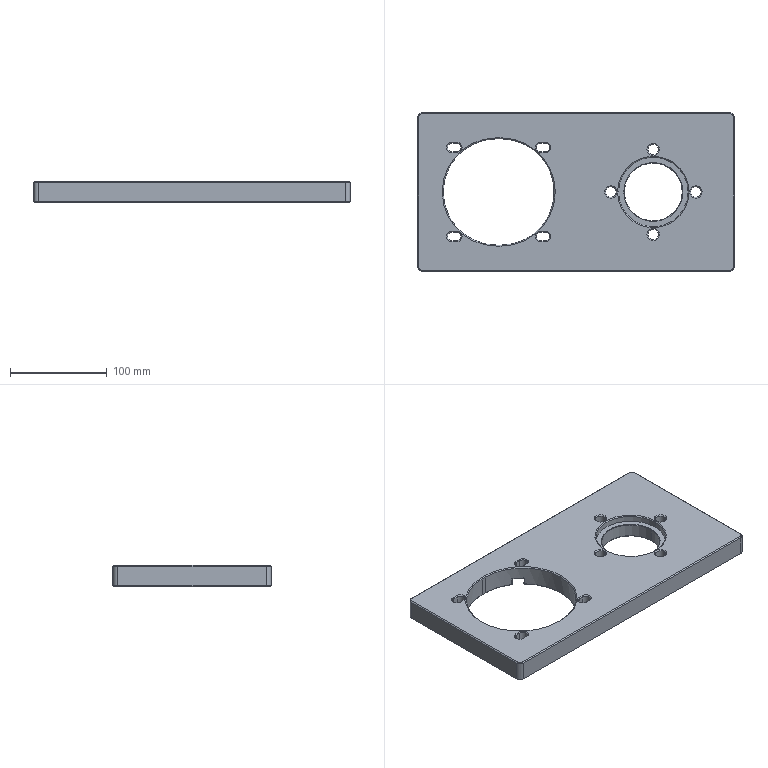NC program | NX | posted with a generic post | part box 328 x 164 x 22 mm
Lines 576 to 1496 of 34171:
(ZLEVEL_PROFILE , TOOL : D10C)
N1114 T10 M6
N1116 G54
N1118 G17 G0 G90 X-156.183 Y-88.046 S3000 M3
N1120 G43 Z30. H10
N1122 Z-0.2
N1124 G94 G1 X-156.442 Y-87.598 F1000.
N1126 G3 X-157.308 Y-87.098 R1.
N1128 G1 X-158.411 Y-87.097 F2500.
N1130 X-159.018 Y-87.098
N1132 G2 X-159.404 Y-87.086 R6.025
N1134 X-161.156 Y-86.864 R10.554
N1136 X-162.064 Y-86.628 R8.203
N1138 X-164.236 Y-85.646 R11.894
N1140 X-166.079 Y-84.217 R12.772
N1142 X-167.162 Y-82.943 R12.307
N1144 X-168.677 Y-79.888 R10.15
N1146 X-168.99 Y-78.466 R11.198
N1148 X-169.095 Y-77.225 R11.169
N1150 G1 X-169.098 Y-77.009
N1152 X-169.097 Y-76.411
N1154 X-169.098 Y-75.308
N1156 G3 X-169.598 Y-74.442 R1.
N1158 G1 X-170.046 Y-74.183
N1160 G0 X-170.044 Y-74.184 Z-0.4
N1162 G1 X-169.598 Y-74.442 F1000.
N1164 G2 X-169.098 Y-75.308 R1.
N1166 G1 Y-76.411 F2500.
N1168 Y-77.009
N1170 X-169.095 Y-77.225
N1172 G3 X-168.99 Y-78.466 R11.058
N1174 X-168.623 Y-80.081 R11.695
N1176 X-167.566 Y-82.362 R11.521
N1178 X-166.082 Y-84.214 R12.251
N1180 X-164.244 Y-85.641 R12.686
N1182 X-161.895 Y-86.683 R11.814
N1184 X-159.957 Y-87.051 R11.645
N1186 X-159.018 Y-87.098 R11.073
N1188 G1 X-158.411
N1190 X-157.308
N1192 G2 X-156.442 Y-87.598 R1.
N1194 G1 X-156.184 Y-88.044
N1196 G0 Z-0.6
N1198 G1 X-156.442 Y-87.598 F1000.
N1200 G3 X-157.308 Y-87.098 R1.
N1202 G1 X-158.411 F2500.
N1204 X-159.018
N1206 G2 X-159.957 Y-87.051 R14.074
N1208 X-161.902 Y-86.681 R11.595
N1210 X-164.25 Y-85.636 R11.748
N1212 X-166.085 Y-84.21 R12.605
N1214 X-167.569 Y-82.358 R12.194
N1216 X-168.625 Y-80.075 R11.466
N1218 X-168.99 Y-78.466 R11.642
N1220 X-169.095 Y-77.225 R10.949
N1222 G1 X-169.098 Y-77.009
N1224 Y-76.411
N1226 Y-75.308
N1228 G3 X-169.598 Y-74.442 R1.
N1230 G1 X-170.042 Y-74.186
N1232 G0 X-170.04 Z-0.8
N1234 G1 X-169.598 Y-74.442 F1000.
N1236 G2 X-169.098 Y-75.308 R1.
N1238 G1 Y-76.411 F2500.
N1240 Y-77.009
N1242 X-169.095 Y-77.225
N1244 G3 X-168.99 Y-78.466 R10.843
N1246 X-168.627 Y-80.068 R11.587
N1248 X-167.571 Y-82.354 R11.409
N1250 X-166.088 Y-84.207 R12.139
N1252 X-164.253 Y-85.634 R12.538
N1254 X-161.912 Y-86.678 R11.716
N1256 X-159.957 Y-87.051 R11.529
N1258 X-159.018 Y-87.098 R13.502
N1260 G1 X-158.411
N1262 X-157.308
N1264 G2 X-156.442 Y-87.598 R1.
N1266 G1 X-156.186 Y-88.04
N1268 G0 X-156.154 Y-88.096 Z-1.
N1270 G1 X-156.442 Y-87.598 F1000.
N1272 G3 X-157.308 Y-87.098 R1.
N1274 G1 X-158.411 F2500.
N1276 X-159.018
N1278 G2 X-169.098 Y-77.009 R10.098
N1280 G1 Y-76.411
N1282 Y-75.308
N1284 G3 X-169.598 Y-74.442 R1.
N1286 G1 X-170.098 Y-74.153
N1288 G0 X-170.1 Y-74.149 Z-1.2
N1290 G1 X-169.596 Y-74.441 F1000.
N1292 G2 X-169.098 Y-75.308 R1.
N1294 G1 X-169.1 Y-76.632 F2500.
N1296 Y-77.
N1298 G3 X-159. Y-87.1 R10.1
N1300 G1 X-158.632
N1302 X-157.308 Y-87.098
N1304 G2 X-156.441 Y-87.596 R1.
N1306 G1 X-156.149 Y-88.1
N1308 G0 Z-1.4
N1310 G1 X-156.441 Y-87.596 F1000.
N1312 G3 X-157.308 Y-87.098 R1.
N1314 G1 X-158.632 Y-87.1 F2500.
N1316 X-159.
N1318 G2 X-169.1 Y-77. R10.1
N1320 G1 Y-76.632
N1322 X-169.098 Y-75.308
N1324 G3 X-169.596 Y-74.441 R1.
N1326 G1 X-170.1 Y-74.149
N1328 G0 Z-1.6
N1330 G1 X-169.596 Y-74.441 F1000.
N1332 G2 X-169.098 Y-75.308 R1.
N1334 G1 X-169.1 Y-76.632 F2500.
N1336 Y-77.
N1338 G3 X-159. Y-87.1 R10.1
N1340 G1 X-158.632
N1342 X-157.308 Y-87.098
N1344 G2 X-156.441 Y-87.596 R1.
N1346 G1 X-156.149 Y-88.1
N1348 G0 Z-1.8
N1350 G1 X-156.441 Y-87.596 F1000.
N1352 G3 X-157.308 Y-87.098 R1.
N1354 G1 X-158.632 Y-87.1 F2500.
N1356 X-159.
N1358 G2 X-169.1 Y-77. R10.1
N1360 G1 Y-76.632
N1362 X-169.098 Y-75.308
N1364 G3 X-169.596 Y-74.441 R1.
N1366 G1 X-170.1 Y-74.149
N1368 G0 Z-2.
N1370 G1 X-169.596 Y-74.441 F1000.
N1372 G2 X-169.098 Y-75.308 R1.
N1374 G1 X-169.1 Y-76.632 F2500.
N1376 Y-77.
N1378 G3 X-159. Y-87.1 R10.1
N1380 G1 X-158.632
N1382 X-157.308 Y-87.098
N1384 G2 X-156.441 Y-87.596 R1.
N1386 G1 X-156.149 Y-88.1
N1388 G0 Z-2.2
N1390 G1 X-156.441 Y-87.596 F1000.
N1392 G3 X-157.308 Y-87.098 R1.
N1394 G1 X-158.632 Y-87.1 F2500.
N1396 X-159.
N1398 G2 X-169.1 Y-77. R10.1
N1400 G1 Y-76.632
N1402 X-169.098 Y-75.308
N1404 G3 X-169.596 Y-74.441 R1.
N1406 G1 X-170.1 Y-74.149
N1408 G0 Z-2.4
N1410 G1 X-169.596 Y-74.441 F1000.
N1412 G2 X-169.098 Y-75.308 R1.
N1414 G1 X-169.1 Y-76.632 F2500.
N1416 Y-77.
N1418 G3 X-159. Y-87.1 R10.1
N1420 G1 X-158.632
N1422 X-157.308 Y-87.098
N1424 G2 X-156.441 Y-87.596 R1.
N1426 G1 X-156.149 Y-88.1
N1428 G0 Z-2.6
N1430 G1 X-156.441 Y-87.596 F1000.
N1432 G3 X-157.308 Y-87.098 R1.
N1434 G1 X-158.632 Y-87.1 F2500.
N1436 X-159.
N1438 G2 X-169.1 Y-77. R10.1
N1440 G1 Y-76.632
N1442 X-169.098 Y-75.308
N1444 G3 X-169.596 Y-74.441 R1.
N1446 G1 X-170.1 Y-74.149
N1448 G0 Z-2.8
N1450 G1 X-169.596 Y-74.441 F1000.
N1452 G2 X-169.098 Y-75.308 R1.
N1454 G1 X-169.1 Y-76.632 F2500.
N1456 Y-77.
N1458 G3 X-159. Y-87.1 R10.1
N1460 G1 X-158.632
N1462 X-157.308 Y-87.098
N1464 G2 X-156.441 Y-87.596 R1.
N1466 G1 X-156.149 Y-88.1
N1468 G0 Z-3.
N1470 G1 X-156.441 Y-87.596 F1000.
N1472 G3 X-157.308 Y-87.098 R1.
N1474 G1 X-158.632 Y-87.1 F2500.
N1476 X-159.
N1478 G2 X-169.1 Y-77. R10.1
N1480 G1 Y-76.632
N1482 X-169.098 Y-75.308
N1484 G3 X-169.596 Y-74.441 R1.
N1486 G1 X-170.1 Y-74.149
N1488 G0 Z-3.2
N1490 G1 X-169.596 Y-74.441 F1000.
N1492 G2 X-169.098 Y-75.308 R1.
N1494 G1 X-169.1 Y-76.632 F2500.
N1496 Y-77.
N1498 G3 X-159. Y-87.1 R10.1
N1500 G1 X-158.632
N1502 X-157.308 Y-87.098
N1504 G2 X-156.441 Y-87.596 R1.
N1506 G1 X-156.149 Y-88.1
N1508 G0 Z-3.4
N1510 G1 X-156.441 Y-87.596 F1000.
N1512 G3 X-157.308 Y-87.098 R1.
N1514 G1 X-158.632 Y-87.1 F2500.
N1516 X-159.
N1518 G2 X-169.1 Y-77. R10.1
N1520 G1 Y-76.632
N1522 X-169.098 Y-75.308
N1524 G3 X-169.596 Y-74.441 R1.
N1526 G1 X-170.1 Y-74.149
N1528 G0 Z-3.6
N1530 G1 X-169.596 Y-74.441 F1000.
N1532 G2 X-169.098 Y-75.308 R1.
N1534 G1 X-169.1 Y-76.632 F2500.
N1536 Y-77.
N1538 G3 X-159. Y-87.1 R10.1
N1540 G1 X-158.632
N1542 X-157.308 Y-87.098
N1544 G2 X-156.441 Y-87.596 R1.
N1546 G1 X-156.149 Y-88.1
N1548 G0 Z-3.8
N1550 G1 X-156.441 Y-87.596 F1000.
N1552 G3 X-157.308 Y-87.098 R1.
N1554 G1 X-158.632 Y-87.1 F2500.
N1556 X-159.
N1558 G2 X-169.1 Y-77. R10.1
N1560 G1 Y-76.632
N1562 X-169.098 Y-75.308
N1564 G3 X-169.596 Y-74.441 R1.
N1566 G1 X-170.1 Y-74.149
N1568 G0 Z-4.
N1570 G1 X-169.596 Y-74.441 F1000.
N1572 G2 X-169.098 Y-75.308 R1.
N1574 G1 X-169.1 Y-76.632 F2500.
N1576 Y-77.
N1578 G3 X-159. Y-87.1 R10.1
N1580 G1 X-158.632
N1582 X-157.308 Y-87.098
N1584 G2 X-156.441 Y-87.596 R1.
N1586 G1 X-156.149 Y-88.1
N1588 G0 Z-4.2
N1590 G1 X-156.441 Y-87.596 F1000.
N1592 G3 X-157.308 Y-87.098 R1.
N1594 G1 X-158.632 Y-87.1 F2500.
N1596 X-159.
N1598 G2 X-169.1 Y-77. R10.1
N1600 G1 Y-76.632
N1602 X-169.098 Y-75.308
N1604 G3 X-169.596 Y-74.441 R1.
N1606 G1 X-170.1 Y-74.149
N1608 G0 Z-4.4
N1610 G1 X-169.596 Y-74.441 F1000.
N1612 G2 X-169.098 Y-75.308 R1.
N1614 G1 X-169.1 Y-76.632 F2500.
N1616 Y-77.
N1618 G3 X-159. Y-87.1 R10.1
N1620 G1 X-158.632
N1622 X-157.308 Y-87.098
N1624 G2 X-156.441 Y-87.596 R1.
N1626 G1 X-156.149 Y-88.1
N1628 G0 Z-4.6
N1630 G1 X-156.441 Y-87.596 F1000.
N1632 G3 X-157.308 Y-87.098 R1.
N1634 G1 X-158.632 Y-87.1 F2500.
N1636 X-159.
N1638 G2 X-169.1 Y-77. R10.1
N1640 G1 Y-76.632
N1642 X-169.098 Y-75.308
N1644 G3 X-169.596 Y-74.441 R1.
N1646 G1 X-170.1 Y-74.149
N1648 G0 Z-4.8
N1650 G1 X-169.596 Y-74.441 F1000.
N1652 G2 X-169.098 Y-75.308 R1.
N1654 G1 X-169.1 Y-76.632 F2500.
N1656 Y-77.
N1658 G3 X-159. Y-87.1 R10.1
N1660 G1 X-158.632
N1662 X-157.308 Y-87.098
N1664 G2 X-156.441 Y-87.596 R1.
N1666 G1 X-156.149 Y-88.1
N1668 G0 Z-5.
N1670 G1 X-156.441 Y-87.596 F1000.
N1672 G3 X-157.308 Y-87.098 R1.
N1674 G1 X-158.632 Y-87.1 F2500.
N1676 X-159.
N1678 G2 X-169.1 Y-77. R10.1
N1680 G1 Y-76.632
N1682 X-169.098 Y-75.308
N1684 G3 X-169.596 Y-74.441 R1.
N1686 G1 X-170.1 Y-74.149
N1688 G0 Z-5.2
N1690 G1 X-169.596 Y-74.441 F1000.
N1692 G2 X-169.098 Y-75.308 R1.
N1694 G1 X-169.1 Y-76.632 F2500.
N1696 Y-77.
N1698 G3 X-159. Y-87.1 R10.1
N1700 G1 X-158.632
N1702 X-157.308 Y-87.098
N1704 G2 X-156.441 Y-87.596 R1.
N1706 G1 X-156.149 Y-88.1
N1708 G0 Z-5.4
N1710 G1 X-156.441 Y-87.596 F1000.
N1712 G3 X-157.308 Y-87.098 R1.
N1714 G1 X-158.632 Y-87.1 F2500.
N1716 X-159.
N1718 G2 X-169.1 Y-77. R10.1
N1720 G1 Y-76.632
N1722 X-169.098 Y-75.308
N1724 G3 X-169.596 Y-74.441 R1.
N1726 G1 X-170.1 Y-74.149
N1728 G0 Z-5.6
N1730 G1 X-169.596 Y-74.441 F1000.
N1732 G2 X-169.098 Y-75.308 R1.
N1734 G1 X-169.1 Y-76.632 F2500.
N1736 Y-77.
N1738 G3 X-159. Y-87.1 R10.1
N1740 G1 X-158.632
N1742 X-157.308 Y-87.098
N1744 G2 X-156.441 Y-87.596 R1.
N1746 G1 X-156.149 Y-88.1
N1748 G0 Z-5.8
N1750 G1 X-156.441 Y-87.596 F1000.
N1752 G3 X-157.308 Y-87.098 R1.
N1754 G1 X-158.632 Y-87.1 F2500.
N1756 X-159.
N1758 G2 X-169.1 Y-77. R10.1
N1760 G1 Y-76.632
N1762 X-169.098 Y-75.308
N1764 G3 X-169.596 Y-74.441 R1.
N1766 G1 X-170.1 Y-74.149
N1768 G0 Z-6.
N1770 G1 X-169.596 Y-74.441 F1000.
N1772 G2 X-169.098 Y-75.308 R1.
N1774 G1 X-169.1 Y-76.632 F2500.
N1776 Y-77.
N1778 G3 X-159. Y-87.1 R10.1
N1780 G1 X-158.632
N1782 X-157.308 Y-87.098
N1784 G2 X-156.441 Y-87.596 R1.
N1786 G1 X-156.149 Y-88.1
N1788 G0 Z-6.2
N1790 G1 X-156.441 Y-87.596 F1000.
N1792 G3 X-157.308 Y-87.098 R1.
N1794 G1 X-158.632 Y-87.1 F2500.
N1796 X-159.
N1798 G2 X-169.1 Y-77. R10.1
N1800 G1 Y-76.632
N1802 X-169.098 Y-75.308
N1804 G3 X-169.596 Y-74.441 R1.
N1806 G1 X-170.1 Y-74.149
N1808 G0 Z-6.4
N1810 G1 X-169.596 Y-74.441 F1000.
N1812 G2 X-169.098 Y-75.308 R1.
N1814 G1 X-169.1 Y-76.632 F2500.
N1816 Y-77.
N1818 G3 X-159. Y-87.1 R10.1
N1820 G1 X-158.632
N1822 X-157.308 Y-87.098
N1824 G2 X-156.441 Y-87.596 R1.
N1826 G1 X-156.149 Y-88.1
N1828 G0 Z-6.6
N1830 G1 X-156.441 Y-87.596 F1000.
N1832 G3 X-157.308 Y-87.098 R1.
N1834 G1 X-158.632 Y-87.1 F2500.
N1836 X-159.
N1838 G2 X-169.1 Y-77. R10.1
N1840 G1 Y-76.632
N1842 X-169.098 Y-75.308
N1844 G3 X-169.596 Y-74.441 R1.
N1846 G1 X-170.1 Y-74.149
N1848 G0 Z-6.8
N1850 G1 X-169.596 Y-74.441 F1000.
N1852 G2 X-169.098 Y-75.308 R1.
N1854 G1 X-169.1 Y-76.632 F2500.
N1856 Y-77.
N1858 G3 X-159. Y-87.1 R10.1
N1860 G1 X-158.632
N1862 X-157.308 Y-87.098
N1864 G2 X-156.441 Y-87.596 R1.
N1866 G1 X-156.149 Y-88.1
N1868 G0 Z-7.
N1870 G1 X-156.441 Y-87.596 F1000.
N1872 G3 X-157.308 Y-87.098 R1.
N1874 G1 X-158.632 Y-87.1 F2500.
N1876 X-159.
N1878 G2 X-169.1 Y-77. R10.1
N1880 G1 Y-76.632
N1882 X-169.098 Y-75.308
N1884 G3 X-169.596 Y-74.441 R1.
N1886 G1 X-170.1 Y-74.149
N1888 G0 Z-7.2
N1890 G1 X-169.596 Y-74.441 F1000.
N1892 G2 X-169.098 Y-75.308 R1.
N1894 G1 X-169.1 Y-76.632 F2500.
N1896 Y-77.
N1898 G3 X-159. Y-87.1 R10.1
N1900 G1 X-158.632
N1902 X-157.308 Y-87.098
N1904 G2 X-156.441 Y-87.596 R1.
N1906 G1 X-156.149 Y-88.1
N1908 G0 Z-7.4
N1910 G1 X-156.441 Y-87.596 F1000.
N1912 G3 X-157.308 Y-87.098 R1.
N1914 G1 X-158.632 Y-87.1 F2500.
N1916 X-159.
N1918 G2 X-169.1 Y-77. R10.1
N1920 G1 Y-76.632
N1922 X-169.098 Y-75.308
N1924 G3 X-169.596 Y-74.441 R1.
N1926 G1 X-170.1 Y-74.149
N1928 G0 Z-7.6
N1930 G1 X-169.596 Y-74.441 F1000.
N1932 G2 X-169.098 Y-75.308 R1.
N1934 G1 X-169.1 Y-76.632 F2500.
N1936 Y-77.
N1938 G3 X-159. Y-87.1 R10.1
N1940 G1 X-158.632
N1942 X-157.308 Y-87.098
N1944 G2 X-156.441 Y-87.596 R1.
N1946 G1 X-156.149 Y-88.1
N1948 G0 Z-7.8
N1950 G1 X-156.441 Y-87.596 F1000.
N1952 G3 X-157.308 Y-87.098 R1.
N1954 G1 X-158.632 Y-87.1 F2500.
N1956 X-159.
N1958 G2 X-169.1 Y-77. R10.1
N1960 G1 Y-76.632
N1962 X-169.098 Y-75.308
N1964 G3 X-169.596 Y-74.441 R1.
N1966 G1 X-170.1 Y-74.149
N1968 G0 Z-8.
N1970 G1 X-169.596 Y-74.441 F1000.
N1972 G2 X-169.098 Y-75.308 R1.
N1974 G1 X-169.1 Y-76.632 F2500.
N1976 Y-77.
N1978 G3 X-159. Y-87.1 R10.1
N1980 G1 X-158.632
N1982 X-157.308 Y-87.098
N1984 G2 X-156.441 Y-87.596 R1.
N1986 G1 X-156.149 Y-88.1
N1988 G0 Z-8.2
N1990 G1 X-156.441 Y-87.596 F1000.
N1992 G3 X-157.308 Y-87.098 R1.
N1994 G1 X-158.632 Y-87.1 F2500.
N1996 X-159.
N1998 G2 X-169.1 Y-77. R10.1
N2000 G1 Y-76.632
N2002 X-169.098 Y-75.308
N2004 G3 X-169.596 Y-74.441 R1.
N2006 G1 X-170.1 Y-74.149
N2008 G0 Z-8.4
N2010 G1 X-169.596 Y-74.441 F1000.
N2012 G2 X-169.098 Y-75.308 R1.
N2014 G1 X-169.1 Y-76.632 F2500.
N2016 Y-77.
N2018 G3 X-159. Y-87.1 R10.1
N2020 G1 X-158.632
N2022 X-157.308 Y-87.098
N2024 G2 X-156.441 Y-87.596 R1.
N2026 G1 X-156.149 Y-88.1
N2028 G0 Z-8.6
N2030 G1 X-156.441 Y-87.596 F1000.
N2032 G3 X-157.308 Y-87.098 R1.
N2034 G1 X-158.632 Y-87.1 F2500.
N2036 X-159.
N2038 G2 X-169.1 Y-77. R10.1
N2040 G1 Y-76.632
N2042 X-169.098 Y-75.308
N2044 G3 X-169.596 Y-74.441 R1.
N2046 G1 X-170.1 Y-74.149
N2048 G0 Z-8.8
N2050 G1 X-169.596 Y-74.441 F1000.
N2052 G2 X-169.098 Y-75.308 R1.
N2054 G1 X-169.1 Y-76.632 F2500.
N2056 Y-77.
N2058 G3 X-159. Y-87.1 R10.1
N2060 G1 X-158.632
N2062 X-157.308 Y-87.098
N2064 G2 X-156.441 Y-87.596 R1.
N2066 G1 X-156.149 Y-88.1
N2068 G0 Z-9.
N2070 G1 X-156.441 Y-87.596 F1000.
N2072 G3 X-157.308 Y-87.098 R1.
N2074 G1 X-158.632 Y-87.1 F2500.
N2076 X-159.
N2078 G2 X-169.1 Y-77. R10.1
N2080 G1 Y-76.632
N2082 X-169.098 Y-75.308
N2084 G3 X-169.596 Y-74.441 R1.
N2086 G1 X-170.1 Y-74.149
N2088 G0 Z-9.2
N2090 G1 X-169.596 Y-74.441 F1000.
N2092 G2 X-169.098 Y-75.308 R1.
N2094 G1 X-169.1 Y-76.632 F2500.
N2096 Y-77.
N2098 G3 X-159. Y-87.1 R10.1
N2100 G1 X-158.632
N2102 X-157.308 Y-87.098
N2104 G2 X-156.441 Y-87.596 R1.
N2106 G1 X-156.149 Y-88.1
N2108 G0 Z-9.4
N2110 G1 X-156.441 Y-87.596 F1000.
N2112 G3 X-157.308 Y-87.098 R1.
N2114 G1 X-158.632 Y-87.1 F2500.
N2116 X-159.
N2118 G2 X-169.1 Y-77. R10.1
N2120 G1 Y-76.632
N2122 X-169.098 Y-75.308
N2124 G3 X-169.596 Y-74.441 R1.
N2126 G1 X-170.1 Y-74.149
N2128 G0 Z-9.6
N2130 G1 X-169.596 Y-74.441 F1000.
N2132 G2 X-169.098 Y-75.308 R1.
N2134 G1 X-169.1 Y-76.632 F2500.
N2136 Y-77.
N2138 G3 X-159. Y-87.1 R10.1
N2140 G1 X-158.632
N2142 X-157.308 Y-87.098
N2144 G2 X-156.441 Y-87.596 R1.
N2146 G1 X-156.149 Y-88.1
N2148 G0 Z-9.8
N2150 G1 X-156.441 Y-87.596 F1000.
N2152 G3 X-157.308 Y-87.098 R1.
N2154 G1 X-158.632 Y-87.1 F2500.
N2156 X-159.
N2158 G2 X-169.1 Y-77. R10.1
N2160 G1 Y-76.632
N2162 X-169.098 Y-75.308
N2164 G3 X-169.596 Y-74.441 R1.
N2166 G1 X-170.1 Y-74.149
N2168 G0 Z-10.
N2170 G1 X-169.596 Y-74.441 F1000.
N2172 G2 X-169.098 Y-75.308 R1.
N2174 G1 X-169.1 Y-76.632 F2500.
N2176 Y-77.
N2178 G3 X-159. Y-87.1 R10.1
N2180 G1 X-158.632
N2182 X-157.308 Y-87.098
N2184 G2 X-156.441 Y-87.596 R1.
N2186 G1 X-156.149 Y-88.1
N2188 G0 Z-10.2
N2190 G1 X-156.441 Y-87.596 F1000.
N2192 G3 X-157.308 Y-87.098 R1.
N2194 G1 X-158.632 Y-87.1 F2500.
N2196 X-159.
N2198 G2 X-169.1 Y-77. R10.1
N2200 G1 Y-76.632
N2202 X-169.098 Y-75.308
N2204 G3 X-169.596 Y-74.441 R1.
N2206 G1 X-170.1 Y-74.149
N2208 G0 Z-10.4
N2210 G1 X-169.596 Y-74.441 F1000.
N2212 G2 X-169.098 Y-75.308 R1.
N2214 G1 X-169.1 Y-76.632 F2500.
N2216 Y-77.
N2218 G3 X-159. Y-87.1 R10.1
N2220 G1 X-158.632
N2222 X-157.308 Y-87.098
N2224 G2 X-156.441 Y-87.596 R1.
N2226 G1 X-156.149 Y-88.1
N2228 G0 Z-10.6
N2230 G1 X-156.441 Y-87.596 F1000.
N2232 G3 X-157.308 Y-87.098 R1.
N2234 G1 X-158.632 Y-87.1 F2500.
N2236 X-159.
N2238 G2 X-169.1 Y-77. R10.1
N2240 G1 Y-76.632
N2242 X-169.098 Y-75.308
N2244 G3 X-169.596 Y-74.441 R1.
N2246 G1 X-170.1 Y-74.149
N2248 G0 Z-10.8
N2250 G1 X-169.596 Y-74.441 F1000.
N2252 G2 X-169.098 Y-75.308 R1.
N2254 G1 X-169.1 Y-76.632 F2500.
N2256 Y-77.
N2258 G3 X-159. Y-87.1 R10.1
N2260 G1 X-158.632
N2262 X-157.308 Y-87.098
N2264 G2 X-156.441 Y-87.596 R1.
N2266 G1 X-156.149 Y-88.1
N2268 G0 Z-11.
N2270 G1 X-156.441 Y-87.596 F1000.
N2272 G3 X-157.308 Y-87.098 R1.
N2274 G1 X-158.632 Y-87.1 F2500.
N2276 X-159.
N2278 G2 X-169.1 Y-77. R10.1
N2280 G1 Y-76.632
N2282 X-169.098 Y-75.308
N2284 G3 X-169.596 Y-74.441 R1.
N2286 G1 X-170.1 Y-74.149
N2288 G0 Z-11.2
N2290 G1 X-169.596 Y-74.441 F1000.
N2292 G2 X-169.098 Y-75.308 R1.
N2294 G1 X-169.1 Y-76.632 F2500.
N2296 Y-77.
N2298 G3 X-159. Y-87.1 R10.1
N2300 G1 X-158.632
N2302 X-157.308 Y-87.098
N2304 G2 X-156.441 Y-87.596 R1.
N2306 G1 X-156.149 Y-88.1
N2308 G0 Z-11.4
N2310 G1 X-156.441 Y-87.597 F1000.
N2312 G3 X-157.308 Y-87.098 R1.
N2314 G1 X-158.632 Y-87.1 F2500.
N2316 X-159.
N2318 G2 X-169.1 Y-77. R10.1
N2320 G1 Y-76.632
N2322 X-169.098 Y-75.308
N2324 G3 X-169.597 Y-74.441 R1.
N2326 G1 X-170.1 Y-74.149
N2328 G0 Z-11.6
N2330 G1 X-169.597 Y-74.441 F1000.
N2332 G2 X-169.098 Y-75.308 R1.
N2334 G1 X-169.1 Y-76.632 F2500.
N2336 Y-77.
N2338 G3 X-159. Y-87.1 R10.1
N2340 G1 X-158.632
N2342 X-157.308 Y-87.098
N2344 G2 X-156.441 Y-87.597 R1.
N2346 G1 X-156.149 Y-88.1
N2348 G0 Z-11.8
N2350 G1 X-156.441 Y-87.597 F1000.
N2352 G3 X-157.308 Y-87.098 R1.
N2354 G1 X-158.632 Y-87.1 F2500.
N2356 X-159.
N2358 G2 X-169.1 Y-77. R10.1
N2360 G1 Y-76.632
N2362 X-169.098 Y-75.308
N2364 G3 X-169.597 Y-74.441 R1.
N2366 G1 X-170.1 Y-74.149
N2368 G0 Z-12.
N2370 G1 X-169.597 Y-74.441 F1000.
N2372 G2 X-169.098 Y-75.308 R1.
N2374 G1 X-169.1 Y-76.632 F2500.
N2376 Y-77.
N2378 G3 X-159. Y-87.1 R10.1
N2380 G1 X-158.632
N2382 X-157.308 Y-87.098
N2384 G2 X-156.441 Y-87.597 R1.
N2386 G1 X-156.149 Y-88.1
N2388 G0 Z-12.2
N2390 G1 X-156.441 Y-87.597 F1000.
N2392 G3 X-157.308 Y-87.098 R1.
N2394 G1 X-158.632 Y-87.1 F2500.
N2396 X-159.
N2398 G2 X-169.1 Y-77. R10.1
N2400 G1 Y-76.632
N2402 X-169.098 Y-75.308
N2404 G3 X-169.597 Y-74.441 R1.
N2406 G1 X-170.1 Y-74.149
N2408 G0 Z-12.4
N2410 G1 X-169.597 Y-74.441 F1000.
N2412 G2 X-169.098 Y-75.308 R1.
N2414 G1 X-169.1 Y-76.632 F2500.
N2416 Y-77.
N2418 G3 X-159. Y-87.1 R10.1
N2420 G1 X-158.632
N2422 X-157.308 Y-87.098
N2424 G2 X-156.441 Y-87.597 R1.
N2426 G1 X-156.149 Y-88.1
N2428 G0 Z-12.6
N2430 G1 X-156.441 Y-87.597 F1000.
N2432 G3 X-157.308 Y-87.098 R1.
N2434 G1 X-158.632 Y-87.1 F2500.
N2436 X-159.
N2438 G2 X-169.1 Y-77. R10.1
N2440 G1 Y-76.632
N2442 X-169.098 Y-75.308
N2444 G3 X-169.597 Y-74.441 R1.
N2446 G1 X-170.1 Y-74.149
N2448 G0 Z-12.8
N2450 G1 X-169.597 Y-74.441 F1000.
N2452 G2 X-169.098 Y-75.308 R1.
N2454 G1 X-169.1 Y-76.632 F2500.
N2456 Y-77.
N2458 G3 X-159. Y-87.1 R10.1
N2460 G1 X-158.632
N2462 X-157.308 Y-87.098
N2464 G2 X-156.441 Y-87.597 R1.
N2466 G1 X-156.149 Y-88.1
N2468 G0 Z-13.
N2470 G1 X-156.441 Y-87.597 F1000.
N2472 G3 X-157.308 Y-87.098 R1.
N2474 G1 X-158.632 Y-87.1 F2500.
N2476 X-159.
N2478 G2 X-169.1 Y-77. R10.1
N2480 G1 Y-76.632
N2482 X-169.098 Y-75.308
N2484 G3 X-169.597 Y-74.441 R1.
N2486 G1 X-170.1 Y-74.149
N2488 G0 Z-13.2
N2490 G1 X-169.597 Y-74.441 F1000.
N2492 G2 X-169.098 Y-75.308 R1.
N2494 G1 X-169.1 Y-76.632 F2500.
N2496 Y-77.
N2498 G3 X-159. Y-87.1 R10.1
N2500 G1 X-158.632
N2502 X-157.308 Y-87.098
N2504 G2 X-156.441 Y-87.597 R1.
N2506 G1 X-156.149 Y-88.1
N2508 G0 Z-13.4
N2510 G1 X-156.441 Y-87.597 F1000.
N2512 G3 X-157.308 Y-87.098 R1.
N2514 G1 X-158.632 Y-87.1 F2500.
N2516 X-159.
N2518 G2 X-169.1 Y-77. R10.1
N2520 G1 Y-76.632
N2522 X-169.098 Y-75.308
N2524 G3 X-169.597 Y-74.441 R1.
N2526 G1 X-170.1 Y-74.149
N2528 G0 Z-13.6
N2530 G1 X-169.597 Y-74.441 F1000.
N2532 G2 X-169.098 Y-75.308 R1.
N2534 G1 X-169.1 Y-76.632 F2500.
N2536 Y-77.
N2538 G3 X-159. Y-87.1 R10.1
N2540 G1 X-158.632
N2542 X-157.308 Y-87.098
N2544 G2 X-156.441 Y-87.597 R1.
N2546 G1 X-156.149 Y-88.1
N2548 G0 Z-13.8
N2550 G1 X-156.441 Y-87.597 F1000.
N2552 G3 X-157.308 Y-87.098 R1.
N2554 G1 X-158.632 Y-87.1 F2500.
N2556 X-159.
N2558 G2 X-169.1 Y-77. R10.1
N2560 G1 Y-76.632
N2562 X-169.098 Y-75.308
N2564 G3 X-169.597 Y-74.441 R1.
N2566 G1 X-170.1 Y-74.149
N2568 G0 Z-14.
N2570 G1 X-169.597 Y-74.441 F1000.
N2572 G2 X-169.098 Y-75.308 R1.
N2574 G1 X-169.1 Y-76.632 F2500.
N2576 Y-77.
N2578 G3 X-159. Y-87.1 R10.1
N2580 G1 X-158.632
N2582 X-157.308 Y-87.098
N2584 G2 X-156.441 Y-87.597 R1.
N2586 G1 X-156.149 Y-88.1
N2588 G0 Z-14.2
N2590 G1 X-156.441 Y-87.597 F1000.
N2592 G3 X-157.308 Y-87.098 R1.
N2594 G1 X-158.632 Y-87.1 F2500.
N2596 X-159.
N2598 G2 X-169.1 Y-77. R10.1
N2600 G1 Y-76.632
N2602 X-169.098 Y-75.308
N2604 G3 X-169.597 Y-74.441 R1.
N2606 G1 X-170.1 Y-74.149
N2608 G0 Z-14.4
N2610 G1 X-169.597 Y-74.441 F1000.
N2612 G2 X-169.098 Y-75.308 R1.
N2614 G1 X-169.1 Y-76.632 F2500.
N2616 Y-77.
N2618 G3 X-159. Y-87.1 R10.1
N2620 G1 X-158.632
N2622 X-157.308 Y-87.098
N2624 G2 X-156.441 Y-87.597 R1.
N2626 G1 X-156.149 Y-88.1
N2628 G0 Z-14.6
N2630 G1 X-156.441 Y-87.597 F1000.
N2632 G3 X-157.308 Y-87.098 R1.
N2634 G1 X-158.632 Y-87.1 F2500.
N2636 X-159.
N2638 G2 X-169.1 Y-77. R10.1
N2640 G1 Y-76.632
N2642 X-169.098 Y-75.308
N2644 G3 X-169.597 Y-74.441 R1.
N2646 G1 X-170.1 Y-74.149
N2648 G0 Z-14.8
N2650 G1 X-169.597 Y-74.441 F1000.
N2652 G2 X-169.098 Y-75.308 R1.
N2654 G1 X-169.1 Y-76.632 F2500.
N2656 Y-77.
N2658 G3 X-159. Y-87.1 R10.1
N2660 G1 X-158.632
N2662 X-157.308 Y-87.098
N2664 G2 X-156.441 Y-87.597 R1.
N2666 G1 X-156.149 Y-88.1
N2668 G0 Z-15.
N2670 G1 X-156.441 Y-87.597 F1000.
N2672 G3 X-157.308 Y-87.098 R1.
N2674 G1 X-158.632 Y-87.1 F2500.
N2676 X-159.
N2678 G2 X-169.1 Y-77. R10.1
N2680 G1 Y-76.632
N2682 X-169.098 Y-75.308
N2684 G3 X-169.597 Y-74.441 R1.
N2686 G1 X-170.1 Y-74.149
N2688 G0 Z-15.2
N2690 G1 X-169.597 Y-74.441 F1000.
N2692 G2 X-169.098 Y-75.308 R1.
N2694 G1 X-169.1 Y-76.632 F2500.
N2696 Y-77.
N2698 G3 X-159. Y-87.1 R10.1
N2700 G1 X-158.632
N2702 X-157.308 Y-87.098
N2704 G2 X-156.441 Y-87.597 R1.
N2706 G1 X-156.149 Y-88.1
N2708 G0 Z-15.4
N2710 G1 X-156.441 Y-87.597 F1000.
N2712 G3 X-157.308 Y-87.098 R1.
N2714 G1 X-158.632 Y-87.1 F2500.
N2716 X-159.
N2718 G2 X-169.1 Y-77. R10.1
N2720 G1 Y-76.632
N2722 X-169.098 Y-75.308
N2724 G3 X-169.597 Y-74.441 R1.
N2726 G1 X-170.1 Y-74.149
N2728 G0 Z-15.6
N2730 G1 X-169.597 Y-74.441 F1000.
N2732 G2 X-169.098 Y-75.308 R1.
N2734 G1 X-169.1 Y-76.632 F2500.
N2736 Y-77.
N2738 G3 X-159. Y-87.1 R10.1
N2740 G1 X-158.632
N2742 X-157.308 Y-87.098
N2744 G2 X-156.441 Y-87.597 R1.
N2746 G1 X-156.149 Y-88.1
N2748 G0 Z-15.8
N2750 G1 X-156.441 Y-87.597 F1000.
N2752 G3 X-157.308 Y-87.098 R1.
N2754 G1 X-158.632 Y-87.1 F2500.
N2756 X-159.
N2758 G2 X-169.1 Y-77. R10.1
N2760 G1 Y-76.632
N2762 X-169.098 Y-75.308
N2764 G3 X-169.597 Y-74.441 R1.
N2766 G1 X-170.1 Y-74.149
N2768 G0 Z-16.
N2770 G1 X-169.597 Y-74.441 F1000.
N2772 G2 X-169.098 Y-75.308 R1.
N2774 G1 X-169.1 Y-76.632 F2500.
N2776 Y-77.
N2778 G3 X-159. Y-87.1 R10.1
N2780 G1 X-158.632
N2782 X-157.308 Y-87.098
N2784 G2 X-156.441 Y-87.597 R1.
N2786 G1 X-156.149 Y-88.1
N2788 G0 Z-16.2
N2790 G1 X-156.441 Y-87.597 F1000.
N2792 G3 X-157.308 Y-87.098 R1.
N2794 G1 X-158.632 Y-87.1 F2500.
N2796 X-159.
N2798 G2 X-169.1 Y-77. R10.1
N2800 G1 Y-76.632
N2802 X-169.098 Y-75.308
N2804 G3 X-169.597 Y-74.441 R1.
N2806 G1 X-170.1 Y-74.149
N2808 G0 Z-16.4
N2810 G1 X-169.597 Y-74.441 F1000.
N2812 G2 X-169.098 Y-75.308 R1.
N2814 G1 X-169.1 Y-76.632 F2500.
N2816 Y-77.
N2818 G3 X-159. Y-87.1 R10.1
N2820 G1 X-158.632
N2822 X-157.308 Y-87.098
N2824 G2 X-156.441 Y-87.597 R1.
N2826 G1 X-156.149 Y-88.1
N2828 G0 Z-16.6
N2830 G1 X-156.441 Y-87.597 F1000.
N2832 G3 X-157.308 Y-87.098 R1.
N2834 G1 X-158.632 Y-87.1 F2500.
N2836 X-159.
N2838 G2 X-169.1 Y-77. R10.1
N2840 G1 Y-76.632
N2842 X-169.098 Y-75.308
N2844 G3 X-169.597 Y-74.441 R1.
N2846 G1 X-170.1 Y-74.149
N2848 G0 Z-16.8
N2850 G1 X-169.597 Y-74.441 F1000.
N2852 G2 X-169.098 Y-75.308 R1.
N2854 G1 X-169.1 Y-76.632 F2500.
N2856 Y-77.
N2858 G3 X-159. Y-87.1 R10.1
N2860 G1 X-158.632
N2862 X-157.308 Y-87.098
N2864 G2 X-156.441 Y-87.597 R1.
N2866 G1 X-156.149 Y-88.1
N2868 G0 Z-17.
N2870 G1 X-156.441 Y-87.597 F1000.
N2872 G3 X-157.308 Y-87.098 R1.
N2874 G1 X-158.632 Y-87.1 F2500.
N2876 X-159.
N2878 G2 X-169.1 Y-77. R10.1
N2880 G1 Y-76.632
N2882 X-169.098 Y-75.308
N2884 G3 X-169.597 Y-74.441 R1.
N2886 G1 X-170.1 Y-74.149
N2888 G0 Z-17.2
N2890 G1 X-169.597 Y-74.441 F1000.
N2892 G2 X-169.098 Y-75.308 R1.
N2894 G1 X-169.1 Y-76.632 F2500.
N2896 Y-77.
N2898 G3 X-159. Y-87.1 R10.1
N2900 G1 X-158.632
N2902 X-157.308 Y-87.098
N2904 G2 X-156.441 Y-87.597 R1.
N2906 G1 X-156.149 Y-88.1
N2908 G0 Z-17.4
N2910 G1 X-156.441 Y-87.597 F1000.
N2912 G3 X-157.308 Y-87.098 R1.
N2914 G1 X-158.632 Y-87.1 F2500.
N2916 X-159.
N2918 G2 X-169.1 Y-77. R10.1
N2920 G1 Y-76.632
N2922 X-169.098 Y-75.308
N2924 G3 X-169.597 Y-74.441 R1.
N2926 G1 X-170.1 Y-74.149
N2928 G0 Z-17.6
N2930 G1 X-169.597 Y-74.441 F1000.
N2932 G2 X-169.098 Y-75.308 R1.
N2934 G1 X-169.1 Y-76.632 F2500.
N2936 Y-77.
N2938 G3 X-159. Y-87.1 R10.1
N2940 G1 X-158.632
N2942 X-157.308 Y-87.098
N2944 G2 X-156.441 Y-87.597 R1.
N2946 G1 X-156.149 Y-88.1
N2948 G0 Z-17.8